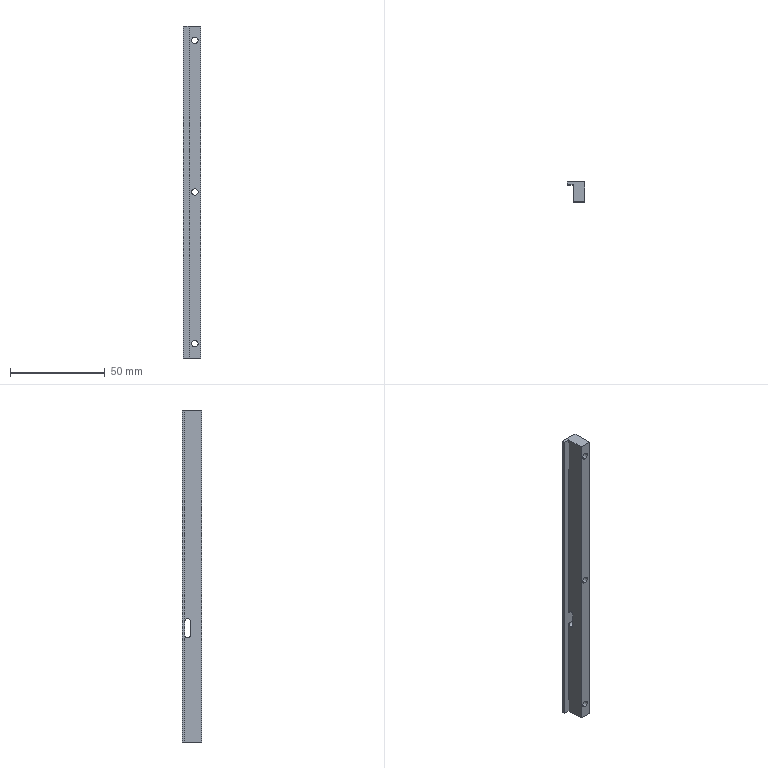Part | STEP file | PN_0021 | 1 solid | 19 faces | box 9 x 10.5 x 175 mm | volume 11358 mm3 | cylinder 10 | plane 9 | commonest cylinder face diameters 3.4 x6 3 x4
STEP:
#1=CARTESIAN_POINT('',(0.,0.,0.));
#2=DIRECTION('',(0.,0.,1.));
#3=DIRECTION('',(1.,0.,0.));
#4=AXIS2_PLACEMENT_3D('',#1,#2,#3);
#5=CARTESIAN_POINT('',(1.5,0.,-78.3));
#6=VERTEX_POINT('',#5);
#7=CARTESIAN_POINT('',(1.5,10.5,-78.3));
#8=VERTEX_POINT('',#7);
#9=CARTESIAN_POINT('',(1.5,10.5,-78.3));
#10=DIRECTION('',(0.,1.,0.));
#11=VECTOR('',#10,1.);
#12=LINE('',#9,#11);
#13=CARTESIAN_POINT('',(1.5,10.5,-80.));
#14=DIRECTION('',(0.,1.,0.));
#15=DIRECTION('',(0.,0.,1.));
#16=AXIS2_PLACEMENT_3D('',#13,#14,#15);
#17=CYLINDRICAL_SURFACE('',#16,1.7);
#18=CARTESIAN_POINT('',(6.283,0.));
#19=DIRECTION('',(0.,1.));
#20=VECTOR('',#19,1.);
#21=LINE('',#18,#20);
#22=(GEOMETRIC_REPRESENTATION_CONTEXT(2)PARAMETRIC_REPRESENTATION_CONTEXT()REPRESENTATION_CONTEXT('',''));
#23=DEFINITIONAL_REPRESENTATION('',(#21),#22);
#24=PCURVE('',#17,#23);
#25=CARTESIAN_POINT('',(1.5,10.5,-80.));
#26=DIRECTION('',(0.,1.,0.));
#27=DIRECTION('',(0.,0.,1.));
#28=AXIS2_PLACEMENT_3D('',#25,#26,#27);
#29=CYLINDRICAL_SURFACE('',#28,1.7);
#30=CARTESIAN_POINT('',(0.,0.));
#31=DIRECTION('',(0.,1.));
#32=VECTOR('',#31,1.);
#33=LINE('',#30,#32);
#34=(GEOMETRIC_REPRESENTATION_CONTEXT(2)PARAMETRIC_REPRESENTATION_CONTEXT()REPRESENTATION_CONTEXT('',''));
#35=DEFINITIONAL_REPRESENTATION('',(#33),#34);
#36=PCURVE('',#29,#35);
#37=SURFACE_CURVE('',#12,(#24,#36),.PCURVE_S1.);
#38=EDGE_CURVE('',#6,#8,#37,.T.);
#39=ORIENTED_EDGE('',*,*,#38,.T.);
#40=CARTESIAN_POINT('',(1.5,10.5,-81.7));
#41=VERTEX_POINT('',#40);
#42=CARTESIAN_POINT('',(1.5,10.5,-80.));
#43=DIRECTION('',(0.,1.,0.));
#44=DIRECTION('',(0.,0.,1.));
#45=AXIS2_PLACEMENT_3D('',#42,#43,#44);
#46=CIRCLE('',#45,1.7);
#47=CARTESIAN_POINT('',(0.,0.));
#48=DIRECTION('',(1.,0.));
#49=VECTOR('',#48,1.);
#50=LINE('',#47,#49);
#51=(GEOMETRIC_REPRESENTATION_CONTEXT(2)PARAMETRIC_REPRESENTATION_CONTEXT()REPRESENTATION_CONTEXT('',''));
#52=DEFINITIONAL_REPRESENTATION('',(#50),#51);
#53=PCURVE('',#17,#52);
#54=CARTESIAN_POINT('',(0.,10.5,0.));
#55=DIRECTION('',(0.,1.,0.));
#56=DIRECTION('',(0.,0.,1.));
#57=AXIS2_PLACEMENT_3D('',#54,#55,#56);
#58=PLANE('',#57);
#59=CARTESIAN_POINT('',(-80.,1.5));
#60=DIRECTION('',(1.,0.));
#61=AXIS2_PLACEMENT_2D('',#59,#60);
#62=CIRCLE('',#61,1.7);
#63=(GEOMETRIC_REPRESENTATION_CONTEXT(2)PARAMETRIC_REPRESENTATION_CONTEXT()REPRESENTATION_CONTEXT('',''));
#64=DEFINITIONAL_REPRESENTATION('',(#62),#63);
#65=PCURVE('',#58,#64);
#66=SURFACE_CURVE('',#46,(#53,#65),.PCURVE_S1.);
#67=EDGE_CURVE('',#41,#8,#66,.T.);
#68=ORIENTED_EDGE('',*,*,#67,.F.);
#69=CARTESIAN_POINT('',(1.5,0.,-81.7));
#70=VERTEX_POINT('',#69);
#71=CARTESIAN_POINT('',(1.5,10.5,-81.7));
#72=DIRECTION('',(0.,1.,0.));
#73=VECTOR('',#72,1.);
#74=LINE('',#71,#73);
#75=CARTESIAN_POINT('',(3.142,0.));
#76=DIRECTION('',(0.,1.));
#77=VECTOR('',#76,1.);
#78=LINE('',#75,#77);
#79=(GEOMETRIC_REPRESENTATION_CONTEXT(2)PARAMETRIC_REPRESENTATION_CONTEXT()REPRESENTATION_CONTEXT('',''));
#80=DEFINITIONAL_REPRESENTATION('',(#78),#79);
#81=PCURVE('',#17,#80);
#82=CARTESIAN_POINT('',(3.142,0.));
#83=DIRECTION('',(0.,1.));
#84=VECTOR('',#83,1.);
#85=LINE('',#82,#84);
#86=(GEOMETRIC_REPRESENTATION_CONTEXT(2)PARAMETRIC_REPRESENTATION_CONTEXT()REPRESENTATION_CONTEXT('',''));
#87=DEFINITIONAL_REPRESENTATION('',(#85),#86);
#88=PCURVE('',#29,#87);
#89=SURFACE_CURVE('',#74,(#81,#88),.PCURVE_S1.);
#90=EDGE_CURVE('',#70,#41,#89,.T.);
#91=ORIENTED_EDGE('',*,*,#90,.F.);
#92=CARTESIAN_POINT('',(1.5,0.,-80.));
#93=DIRECTION('',(0.,1.,0.));
#94=DIRECTION('',(0.,0.,1.));
#95=AXIS2_PLACEMENT_3D('',#92,#93,#94);
#96=CIRCLE('',#95,1.7);
#97=CARTESIAN_POINT('',(0.,-10.5));
#98=DIRECTION('',(1.,0.));
#99=VECTOR('',#98,1.);
#100=LINE('',#97,#99);
#101=(GEOMETRIC_REPRESENTATION_CONTEXT(2)PARAMETRIC_REPRESENTATION_CONTEXT()REPRESENTATION_CONTEXT('',''));
#102=DEFINITIONAL_REPRESENTATION('',(#100),#101);
#103=PCURVE('',#17,#102);
#104=CARTESIAN_POINT('',(0.,0.,0.));
#105=DIRECTION('',(0.,1.,0.));
#106=DIRECTION('',(0.,0.,1.));
#107=AXIS2_PLACEMENT_3D('',#104,#105,#106);
#108=PLANE('',#107);
#109=CARTESIAN_POINT('',(-80.,1.5));
#110=DIRECTION('',(1.,0.));
#111=AXIS2_PLACEMENT_2D('',#109,#110);
#112=CIRCLE('',#111,1.7);
#113=(GEOMETRIC_REPRESENTATION_CONTEXT(2)PARAMETRIC_REPRESENTATION_CONTEXT()REPRESENTATION_CONTEXT('',''));
#114=DEFINITIONAL_REPRESENTATION('',(#112),#113);
#115=PCURVE('',#108,#114);
#116=SURFACE_CURVE('',#96,(#103,#115),.PCURVE_S1.);
#117=EDGE_CURVE('',#70,#6,#116,.T.);
#118=ORIENTED_EDGE('',*,*,#117,.T.);
#119=EDGE_LOOP('',(#39,#68,#91,#118));
#120=FACE_BOUND('',#119,.F.);
#121=ADVANCED_FACE('',(#120),#17,.F.);
#122=CARTESIAN_POINT('',(1.5,0.,1.7));
#123=VERTEX_POINT('',#122);
#124=CARTESIAN_POINT('',(1.5,10.5,1.7));
#125=VERTEX_POINT('',#124);
#126=CARTESIAN_POINT('',(1.5,10.5,1.7));
#127=DIRECTION('',(0.,1.,0.));
#128=VECTOR('',#127,1.);
#129=LINE('',#126,#128);
#130=CARTESIAN_POINT('',(1.5,10.5,0.));
#131=DIRECTION('',(0.,1.,0.));
#132=DIRECTION('',(0.,0.,1.));
#133=AXIS2_PLACEMENT_3D('',#130,#131,#132);
#134=CYLINDRICAL_SURFACE('',#133,1.7);
#135=CARTESIAN_POINT('',(6.283,0.));
#136=DIRECTION('',(0.,1.));
#137=VECTOR('',#136,1.);
#138=LINE('',#135,#137);
#139=(GEOMETRIC_REPRESENTATION_CONTEXT(2)PARAMETRIC_REPRESENTATION_CONTEXT()REPRESENTATION_CONTEXT('',''));
#140=DEFINITIONAL_REPRESENTATION('',(#138),#139);
#141=PCURVE('',#134,#140);
#142=CARTESIAN_POINT('',(1.5,10.5,0.));
#143=DIRECTION('',(0.,1.,0.));
#144=DIRECTION('',(0.,0.,1.));
#145=AXIS2_PLACEMENT_3D('',#142,#143,#144);
#146=CYLINDRICAL_SURFACE('',#145,1.7);
#147=CARTESIAN_POINT('',(0.,0.));
#148=DIRECTION('',(0.,1.));
#149=VECTOR('',#148,1.);
#150=LINE('',#147,#149);
#151=(GEOMETRIC_REPRESENTATION_CONTEXT(2)PARAMETRIC_REPRESENTATION_CONTEXT()REPRESENTATION_CONTEXT('',''));
#152=DEFINITIONAL_REPRESENTATION('',(#150),#151);
#153=PCURVE('',#146,#152);
#154=SURFACE_CURVE('',#129,(#141,#153),.PCURVE_S1.);
#155=EDGE_CURVE('',#123,#125,#154,.T.);
#156=ORIENTED_EDGE('',*,*,#155,.T.);
#157=CARTESIAN_POINT('',(1.5,10.5,-1.7));
#158=VERTEX_POINT('',#157);
#159=CARTESIAN_POINT('',(1.5,10.5,0.));
#160=DIRECTION('',(0.,1.,0.));
#161=DIRECTION('',(0.,0.,1.));
#162=AXIS2_PLACEMENT_3D('',#159,#160,#161);
#163=CIRCLE('',#162,1.7);
#164=CARTESIAN_POINT('',(0.,0.));
#165=DIRECTION('',(1.,0.));
#166=VECTOR('',#165,1.);
#167=LINE('',#164,#166);
#168=(GEOMETRIC_REPRESENTATION_CONTEXT(2)PARAMETRIC_REPRESENTATION_CONTEXT()REPRESENTATION_CONTEXT('',''));
#169=DEFINITIONAL_REPRESENTATION('',(#167),#168);
#170=PCURVE('',#134,#169);
#171=CARTESIAN_POINT('',(0.,1.5));
#172=DIRECTION('',(1.,0.));
#173=AXIS2_PLACEMENT_2D('',#171,#172);
#174=CIRCLE('',#173,1.7);
#175=(GEOMETRIC_REPRESENTATION_CONTEXT(2)PARAMETRIC_REPRESENTATION_CONTEXT()REPRESENTATION_CONTEXT('',''));
#176=DEFINITIONAL_REPRESENTATION('',(#174),#175);
#177=PCURVE('',#58,#176);
#178=SURFACE_CURVE('',#163,(#170,#177),.PCURVE_S1.);
#179=EDGE_CURVE('',#158,#125,#178,.T.);
#180=ORIENTED_EDGE('',*,*,#179,.F.);
#181=CARTESIAN_POINT('',(1.5,0.,-1.7));
#182=VERTEX_POINT('',#181);
#183=CARTESIAN_POINT('',(1.5,10.5,-1.7));
#184=DIRECTION('',(0.,1.,0.));
#185=VECTOR('',#184,1.);
#186=LINE('',#183,#185);
#187=CARTESIAN_POINT('',(3.142,0.));
#188=DIRECTION('',(0.,1.));
#189=VECTOR('',#188,1.);
#190=LINE('',#187,#189);
#191=(GEOMETRIC_REPRESENTATION_CONTEXT(2)PARAMETRIC_REPRESENTATION_CONTEXT()REPRESENTATION_CONTEXT('',''));
#192=DEFINITIONAL_REPRESENTATION('',(#190),#191);
#193=PCURVE('',#134,#192);
#194=CARTESIAN_POINT('',(3.142,0.));
#195=DIRECTION('',(0.,1.));
#196=VECTOR('',#195,1.);
#197=LINE('',#194,#196);
#198=(GEOMETRIC_REPRESENTATION_CONTEXT(2)PARAMETRIC_REPRESENTATION_CONTEXT()REPRESENTATION_CONTEXT('',''));
#199=DEFINITIONAL_REPRESENTATION('',(#197),#198);
#200=PCURVE('',#146,#199);
#201=SURFACE_CURVE('',#186,(#193,#200),.PCURVE_S1.);
#202=EDGE_CURVE('',#182,#158,#201,.T.);
#203=ORIENTED_EDGE('',*,*,#202,.F.);
#204=CARTESIAN_POINT('',(1.5,0.,0.));
#205=DIRECTION('',(0.,1.,0.));
#206=DIRECTION('',(0.,0.,1.));
#207=AXIS2_PLACEMENT_3D('',#204,#205,#206);
#208=CIRCLE('',#207,1.7);
#209=CARTESIAN_POINT('',(0.,-10.5));
#210=DIRECTION('',(1.,0.));
#211=VECTOR('',#210,1.);
#212=LINE('',#209,#211);
#213=(GEOMETRIC_REPRESENTATION_CONTEXT(2)PARAMETRIC_REPRESENTATION_CONTEXT()REPRESENTATION_CONTEXT('',''));
#214=DEFINITIONAL_REPRESENTATION('',(#212),#213);
#215=PCURVE('',#134,#214);
#216=CARTESIAN_POINT('',(0.,1.5));
#217=DIRECTION('',(1.,0.));
#218=AXIS2_PLACEMENT_2D('',#216,#217);
#219=CIRCLE('',#218,1.7);
#220=(GEOMETRIC_REPRESENTATION_CONTEXT(2)PARAMETRIC_REPRESENTATION_CONTEXT()REPRESENTATION_CONTEXT('',''));
#221=DEFINITIONAL_REPRESENTATION('',(#219),#220);
#222=PCURVE('',#108,#221);
#223=SURFACE_CURVE('',#208,(#215,#222),.PCURVE_S1.);
#224=EDGE_CURVE('',#182,#123,#223,.T.);
#225=ORIENTED_EDGE('',*,*,#224,.T.);
#226=EDGE_LOOP('',(#156,#180,#203,#225));
#227=FACE_BOUND('',#226,.F.);
#228=ADVANCED_FACE('',(#227),#134,.F.);
#229=CARTESIAN_POINT('',(1.5,0.,81.7));
#230=VERTEX_POINT('',#229);
#231=CARTESIAN_POINT('',(1.5,10.5,81.7));
#232=VERTEX_POINT('',#231);
#233=CARTESIAN_POINT('',(1.5,10.5,81.7));
#234=DIRECTION('',(0.,1.,0.));
#235=VECTOR('',#234,1.);
#236=LINE('',#233,#235);
#237=CARTESIAN_POINT('',(1.5,10.5,80.));
#238=DIRECTION('',(0.,1.,0.));
#239=DIRECTION('',(0.,0.,1.));
#240=AXIS2_PLACEMENT_3D('',#237,#238,#239);
#241=CYLINDRICAL_SURFACE('',#240,1.7);
#242=CARTESIAN_POINT('',(6.283,0.));
#243=DIRECTION('',(0.,1.));
#244=VECTOR('',#243,1.);
#245=LINE('',#242,#244);
#246=(GEOMETRIC_REPRESENTATION_CONTEXT(2)PARAMETRIC_REPRESENTATION_CONTEXT()REPRESENTATION_CONTEXT('',''));
#247=DEFINITIONAL_REPRESENTATION('',(#245),#246);
#248=PCURVE('',#241,#247);
#249=CARTESIAN_POINT('',(1.5,10.5,80.));
#250=DIRECTION('',(0.,1.,0.));
#251=DIRECTION('',(0.,0.,1.));
#252=AXIS2_PLACEMENT_3D('',#249,#250,#251);
#253=CYLINDRICAL_SURFACE('',#252,1.7);
#254=CARTESIAN_POINT('',(0.,0.));
#255=DIRECTION('',(0.,1.));
#256=VECTOR('',#255,1.);
#257=LINE('',#254,#256);
#258=(GEOMETRIC_REPRESENTATION_CONTEXT(2)PARAMETRIC_REPRESENTATION_CONTEXT()REPRESENTATION_CONTEXT('',''));
#259=DEFINITIONAL_REPRESENTATION('',(#257),#258);
#260=PCURVE('',#253,#259);
#261=SURFACE_CURVE('',#236,(#248,#260),.PCURVE_S1.);
#262=EDGE_CURVE('',#230,#232,#261,.T.);
#263=ORIENTED_EDGE('',*,*,#262,.T.);
#264=CARTESIAN_POINT('',(1.5,10.5,78.3));
#265=VERTEX_POINT('',#264);
#266=CARTESIAN_POINT('',(1.5,10.5,80.));
#267=DIRECTION('',(0.,1.,0.));
#268=DIRECTION('',(0.,0.,1.));
#269=AXIS2_PLACEMENT_3D('',#266,#267,#268);
#270=CIRCLE('',#269,1.7);
#271=CARTESIAN_POINT('',(0.,0.));
#272=DIRECTION('',(1.,0.));
#273=VECTOR('',#272,1.);
#274=LINE('',#271,#273);
#275=(GEOMETRIC_REPRESENTATION_CONTEXT(2)PARAMETRIC_REPRESENTATION_CONTEXT()REPRESENTATION_CONTEXT('',''));
#276=DEFINITIONAL_REPRESENTATION('',(#274),#275);
#277=PCURVE('',#241,#276);
#278=CARTESIAN_POINT('',(80.,1.5));
#279=DIRECTION('',(1.,0.));
#280=AXIS2_PLACEMENT_2D('',#278,#279);
#281=CIRCLE('',#280,1.7);
#282=(GEOMETRIC_REPRESENTATION_CONTEXT(2)PARAMETRIC_REPRESENTATION_CONTEXT()REPRESENTATION_CONTEXT('',''));
#283=DEFINITIONAL_REPRESENTATION('',(#281),#282);
#284=PCURVE('',#58,#283);
#285=SURFACE_CURVE('',#270,(#277,#284),.PCURVE_S1.);
#286=EDGE_CURVE('',#265,#232,#285,.T.);
#287=ORIENTED_EDGE('',*,*,#286,.F.);
#288=CARTESIAN_POINT('',(1.5,0.,78.3));
#289=VERTEX_POINT('',#288);
#290=CARTESIAN_POINT('',(1.5,10.5,78.3));
#291=DIRECTION('',(0.,1.,0.));
#292=VECTOR('',#291,1.);
#293=LINE('',#290,#292);
#294=CARTESIAN_POINT('',(3.142,0.));
#295=DIRECTION('',(0.,1.));
#296=VECTOR('',#295,1.);
#297=LINE('',#294,#296);
#298=(GEOMETRIC_REPRESENTATION_CONTEXT(2)PARAMETRIC_REPRESENTATION_CONTEXT()REPRESENTATION_CONTEXT('',''));
#299=DEFINITIONAL_REPRESENTATION('',(#297),#298);
#300=PCURVE('',#241,#299);
#301=CARTESIAN_POINT('',(3.142,0.));
#302=DIRECTION('',(0.,1.));
#303=VECTOR('',#302,1.);
#304=LINE('',#301,#303);
#305=(GEOMETRIC_REPRESENTATION_CONTEXT(2)PARAMETRIC_REPRESENTATION_CONTEXT()REPRESENTATION_CONTEXT('',''));
#306=DEFINITIONAL_REPRESENTATION('',(#304),#305);
#307=PCURVE('',#253,#306);
#308=SURFACE_CURVE('',#293,(#300,#307),.PCURVE_S1.);
#309=EDGE_CURVE('',#289,#265,#308,.T.);
#310=ORIENTED_EDGE('',*,*,#309,.F.);
#311=CARTESIAN_POINT('',(1.5,0.,80.));
#312=DIRECTION('',(0.,1.,0.));
#313=DIRECTION('',(0.,0.,1.));
#314=AXIS2_PLACEMENT_3D('',#311,#312,#313);
#315=CIRCLE('',#314,1.7);
#316=CARTESIAN_POINT('',(0.,-10.5));
#317=DIRECTION('',(1.,0.));
#318=VECTOR('',#317,1.);
#319=LINE('',#316,#318);
#320=(GEOMETRIC_REPRESENTATION_CONTEXT(2)PARAMETRIC_REPRESENTATION_CONTEXT()REPRESENTATION_CONTEXT('',''));
#321=DEFINITIONAL_REPRESENTATION('',(#319),#320);
#322=PCURVE('',#241,#321);
#323=CARTESIAN_POINT('',(80.,1.5));
#324=DIRECTION('',(1.,0.));
#325=AXIS2_PLACEMENT_2D('',#323,#324);
#326=CIRCLE('',#325,1.7);
#327=(GEOMETRIC_REPRESENTATION_CONTEXT(2)PARAMETRIC_REPRESENTATION_CONTEXT()REPRESENTATION_CONTEXT('',''));
#328=DEFINITIONAL_REPRESENTATION('',(#326),#327);
#329=PCURVE('',#108,#328);
#330=SURFACE_CURVE('',#315,(#322,#329),.PCURVE_S1.);
#331=EDGE_CURVE('',#289,#230,#330,.T.);
#332=ORIENTED_EDGE('',*,*,#331,.T.);
#333=EDGE_LOOP('',(#263,#287,#310,#332));
#334=FACE_BOUND('',#333,.F.);
#335=ADVANCED_FACE('',(#334),#241,.F.);
#336=CARTESIAN_POINT('',(4.5,6.,-24.));
#337=VERTEX_POINT('',#336);
#338=CARTESIAN_POINT('',(4.5,7.5,-22.5));
#339=VERTEX_POINT('',#338);
#340=CARTESIAN_POINT('',(4.5,7.5,-24.));
#341=DIRECTION('',(-1.,0.,0.));
#342=DIRECTION('',(0.,0.,1.));
#343=AXIS2_PLACEMENT_3D('',#340,#341,#342);
#344=CIRCLE('',#343,1.5);
#345=CARTESIAN_POINT('',(4.5,10.5,-87.5));
#346=DIRECTION('',(-1.,0.,0.));
#347=DIRECTION('',(0.,0.,1.));
#348=AXIS2_PLACEMENT_3D('',#345,#346,#347);
#349=PLANE('',#348);
#350=CARTESIAN_POINT('',(63.5,-3.));
#351=DIRECTION('',(1.,0.));
#352=AXIS2_PLACEMENT_2D('',#350,#351);
#353=CIRCLE('',#352,1.5);
#354=(GEOMETRIC_REPRESENTATION_CONTEXT(2)PARAMETRIC_REPRESENTATION_CONTEXT()REPRESENTATION_CONTEXT('',''));
#355=DEFINITIONAL_REPRESENTATION('',(#353),#354);
#356=PCURVE('',#349,#355);
#357=CARTESIAN_POINT('',(4.5,7.5,-24.));
#358=DIRECTION('',(1.,0.,0.));
#359=DIRECTION('',(0.,0.,-1.));
#360=AXIS2_PLACEMENT_3D('',#357,#358,#359);
#361=CYLINDRICAL_SURFACE('',#360,1.5);
#362=CARTESIAN_POINT('',(9.425,0.));
#363=DIRECTION('',(-1.,0.));
#364=VECTOR('',#363,1.);
#365=LINE('',#362,#364);
#366=(GEOMETRIC_REPRESENTATION_CONTEXT(2)PARAMETRIC_REPRESENTATION_CONTEXT()REPRESENTATION_CONTEXT('',''));
#367=DEFINITIONAL_REPRESENTATION('',(#365),#366);
#368=PCURVE('',#361,#367);
#369=SURFACE_CURVE('',#344,(#356,#368),.PCURVE_S1.);
#370=EDGE_CURVE('',#337,#339,#369,.T.);
#371=ORIENTED_EDGE('',*,*,#370,.T.);
#372=CARTESIAN_POINT('',(4.5,9.,-24.));
#373=VERTEX_POINT('',#372);
#374=CARTESIAN_POINT('',(4.5,7.5,-24.));
#375=DIRECTION('',(-1.,0.,0.));
#376=DIRECTION('',(0.,0.,1.));
#377=AXIS2_PLACEMENT_3D('',#374,#375,#376);
#378=CIRCLE('',#377,1.5);
#379=CARTESIAN_POINT('',(63.5,-3.));
#380=DIRECTION('',(1.,0.));
#381=AXIS2_PLACEMENT_2D('',#379,#380);
#382=CIRCLE('',#381,1.5);
#383=(GEOMETRIC_REPRESENTATION_CONTEXT(2)PARAMETRIC_REPRESENTATION_CONTEXT()REPRESENTATION_CONTEXT('',''));
#384=DEFINITIONAL_REPRESENTATION('',(#382),#383);
#385=PCURVE('',#349,#384);
#386=CARTESIAN_POINT('',(-4.5,7.5,-24.));
#387=DIRECTION('',(1.,0.,0.));
#388=DIRECTION('',(0.,0.,-1.));
#389=AXIS2_PLACEMENT_3D('',#386,#387,#388);
#390=CYLINDRICAL_SURFACE('',#389,1.5);
#391=CARTESIAN_POINT('',(3.142,9.));
#392=DIRECTION('',(-1.,0.));
#393=VECTOR('',#392,1.);
#394=LINE('',#391,#393);
#395=(GEOMETRIC_REPRESENTATION_CONTEXT(2)PARAMETRIC_REPRESENTATION_CONTEXT()REPRESENTATION_CONTEXT('',''));
#396=DEFINITIONAL_REPRESENTATION('',(#394),#395);
#397=PCURVE('',#390,#396);
#398=SURFACE_CURVE('',#378,(#385,#397),.PCURVE_S1.);
#399=EDGE_CURVE('',#339,#373,#398,.T.);
#400=ORIENTED_EDGE('',*,*,#399,.T.);
#401=CARTESIAN_POINT('',(4.5,9.,-31.));
#402=VERTEX_POINT('',#401);
#403=CARTESIAN_POINT('',(4.5,9.,-32.5));
#404=DIRECTION('',(0.,0.,-1.));
#405=VECTOR('',#404,1.);
#406=LINE('',#403,#405);
#407=CARTESIAN_POINT('',(55.,-1.5));
#408=DIRECTION('',(-1.,0.));
#409=VECTOR('',#408,1.);
#410=LINE('',#407,#409);
#411=(GEOMETRIC_REPRESENTATION_CONTEXT(2)PARAMETRIC_REPRESENTATION_CONTEXT()REPRESENTATION_CONTEXT('',''));
#412=DEFINITIONAL_REPRESENTATION('',(#410),#411);
#413=PCURVE('',#349,#412);
#414=CARTESIAN_POINT('',(-4.5,9.,-87.5));
#415=DIRECTION('',(0.,1.,0.));
#416=DIRECTION('',(0.,0.,1.));
#417=AXIS2_PLACEMENT_3D('',#414,#415,#416);
#418=PLANE('',#417);
#419=CARTESIAN_POINT('',(55.,9.));
#420=DIRECTION('',(-1.,0.));
#421=VECTOR('',#420,1.);
#422=LINE('',#419,#421);
#423=(GEOMETRIC_REPRESENTATION_CONTEXT(2)PARAMETRIC_REPRESENTATION_CONTEXT()REPRESENTATION_CONTEXT('',''));
#424=DEFINITIONAL_REPRESENTATION('',(#422),#423);
#425=PCURVE('',#418,#424);
#426=SURFACE_CURVE('',#406,(#413,#425),.PCURVE_S1.);
#427=EDGE_CURVE('',#373,#402,#426,.T.);
#428=ORIENTED_EDGE('',*,*,#427,.T.);
#429=CARTESIAN_POINT('',(4.5,7.5,-32.5));
#430=VERTEX_POINT('',#429);
#431=CARTESIAN_POINT('',(4.5,7.5,-31.));
#432=DIRECTION('',(-1.,0.,0.));
#433=DIRECTION('',(0.,0.,1.));
#434=AXIS2_PLACEMENT_3D('',#431,#432,#433);
#435=CIRCLE('',#434,1.5);
#436=CARTESIAN_POINT('',(56.5,-3.));
#437=DIRECTION('',(1.,0.));
#438=AXIS2_PLACEMENT_2D('',#436,#437);
#439=CIRCLE('',#438,1.5);
#440=(GEOMETRIC_REPRESENTATION_CONTEXT(2)PARAMETRIC_REPRESENTATION_CONTEXT()REPRESENTATION_CONTEXT('',''));
#441=DEFINITIONAL_REPRESENTATION('',(#439),#440);
#442=PCURVE('',#349,#441);
#443=CARTESIAN_POINT('',(4.5,7.5,-31.));
#444=DIRECTION('',(1.,0.,0.));
#445=DIRECTION('',(0.,0.,-1.));
#446=AXIS2_PLACEMENT_3D('',#443,#444,#445);
#447=CYLINDRICAL_SURFACE('',#446,1.5);
#448=CARTESIAN_POINT('',(3.142,0.));
#449=DIRECTION('',(-1.,0.));
#450=VECTOR('',#449,1.);
#451=LINE('',#448,#450);
#452=(GEOMETRIC_REPRESENTATION_CONTEXT(2)PARAMETRIC_REPRESENTATION_CONTEXT()REPRESENTATION_CONTEXT('',''));
#453=DEFINITIONAL_REPRESENTATION('',(#451),#452);
#454=PCURVE('',#447,#453);
#455=SURFACE_CURVE('',#435,(#442,#454),.PCURVE_S1.);
#456=EDGE_CURVE('',#402,#430,#455,.T.);
#457=ORIENTED_EDGE('',*,*,#456,.T.);
#458=CARTESIAN_POINT('',(4.5,6.,-31.));
#459=VERTEX_POINT('',#458);
#460=CARTESIAN_POINT('',(4.5,7.5,-31.));
#461=DIRECTION('',(-1.,0.,0.));
#462=DIRECTION('',(0.,0.,1.));
#463=AXIS2_PLACEMENT_3D('',#460,#461,#462);
#464=CIRCLE('',#463,1.5);
#465=CARTESIAN_POINT('',(56.5,-3.));
#466=DIRECTION('',(1.,0.));
#467=AXIS2_PLACEMENT_2D('',#465,#466);
#468=CIRCLE('',#467,1.5);
#469=(GEOMETRIC_REPRESENTATION_CONTEXT(2)PARAMETRIC_REPRESENTATION_CONTEXT()REPRESENTATION_CONTEXT('',''));
#470=DEFINITIONAL_REPRESENTATION('',(#468),#469);
#471=PCURVE('',#349,#470);
#472=CARTESIAN_POINT('',(4.5,7.5,-31.));
#473=DIRECTION('',(1.,0.,0.));
#474=DIRECTION('',(0.,0.,-1.));
#475=AXIS2_PLACEMENT_3D('',#472,#473,#474);
#476=CYLINDRICAL_SURFACE('',#475,1.5);
#477=CARTESIAN_POINT('',(9.425,0.));
#478=DIRECTION('',(-1.,0.));
#479=VECTOR('',#478,1.);
#480=LINE('',#477,#479);
#481=(GEOMETRIC_REPRESENTATION_CONTEXT(2)PARAMETRIC_REPRESENTATION_CONTEXT()REPRESENTATION_CONTEXT('',''));
#482=DEFINITIONAL_REPRESENTATION('',(#480),#481);
#483=PCURVE('',#476,#482);
#484=SURFACE_CURVE('',#464,(#471,#483),.PCURVE_S1.);
#485=EDGE_CURVE('',#430,#459,#484,.T.);
#486=ORIENTED_EDGE('',*,*,#485,.T.);
#487=CARTESIAN_POINT('',(4.5,6.,-32.5));
#488=DIRECTION('',(0.,0.,1.));
#489=VECTOR('',#488,1.);
#490=LINE('',#487,#489);
#491=CARTESIAN_POINT('',(55.,-4.5));
#492=DIRECTION('',(1.,0.));
#493=VECTOR('',#492,1.);
#494=LINE('',#491,#493);
#495=(GEOMETRIC_REPRESENTATION_CONTEXT(2)PARAMETRIC_REPRESENTATION_CONTEXT()REPRESENTATION_CONTEXT('',''));
#496=DEFINITIONAL_REPRESENTATION('',(#494),#495);
#497=PCURVE('',#349,#496);
#498=CARTESIAN_POINT('',(4.5,6.,-32.5));
#499=DIRECTION('',(0.,-1.,0.));
#500=DIRECTION('',(0.,0.,-1.));
#501=AXIS2_PLACEMENT_3D('',#498,#499,#500);
#502=PLANE('',#501);
#503=CARTESIAN_POINT('',(0.,0.));
#504=DIRECTION('',(-1.,0.));
#505=VECTOR('',#504,1.);
#506=LINE('',#503,#505);
#507=(GEOMETRIC_REPRESENTATION_CONTEXT(2)PARAMETRIC_REPRESENTATION_CONTEXT()REPRESENTATION_CONTEXT('',''));
#508=DEFINITIONAL_REPRESENTATION('',(#506),#507);
#509=PCURVE('',#502,#508);
#510=SURFACE_CURVE('',#490,(#497,#509),.PCURVE_S1.);
#511=EDGE_CURVE('',#459,#337,#510,.T.);
#512=ORIENTED_EDGE('',*,*,#511,.T.);
#513=EDGE_LOOP('',(#371,#400,#428,#457,#486,#512));
#514=FACE_BOUND('',#513,.T.);
#515=CARTESIAN_POINT('',(4.5,0.,87.5));
#516=VERTEX_POINT('',#515);
#517=CARTESIAN_POINT('',(4.5,0.,-87.5));
#518=VERTEX_POINT('',#517);
#519=CARTESIAN_POINT('',(4.5,0.,-87.5));
#520=DIRECTION('',(0.,0.,-1.));
#521=VECTOR('',#520,1.);
#522=LINE('',#519,#521);
#523=CARTESIAN_POINT('',(0.,-10.5));
#524=DIRECTION('',(-1.,0.));
#525=VECTOR('',#524,1.);
#526=LINE('',#523,#525);
#527=(GEOMETRIC_REPRESENTATION_CONTEXT(2)PARAMETRIC_REPRESENTATION_CONTEXT()REPRESENTATION_CONTEXT('',''));
#528=DEFINITIONAL_REPRESENTATION('',(#526),#527);
#529=PCURVE('',#349,#528);
#530=CARTESIAN_POINT('',(-87.5,4.5));
#531=DIRECTION('',(-1.,0.));
#532=VECTOR('',#531,1.);
#533=LINE('',#530,#532);
#534=(GEOMETRIC_REPRESENTATION_CONTEXT(2)PARAMETRIC_REPRESENTATION_CONTEXT()REPRESENTATION_CONTEXT('',''));
#535=DEFINITIONAL_REPRESENTATION('',(#533),#534);
#536=PCURVE('',#108,#535);
#537=SURFACE_CURVE('',#522,(#529,#536),.PCURVE_S1.);
#538=EDGE_CURVE('',#516,#518,#537,.T.);
#539=ORIENTED_EDGE('',*,*,#538,.T.);
#540=CARTESIAN_POINT('',(4.5,10.5,-87.5));
#541=VERTEX_POINT('',#540);
#542=CARTESIAN_POINT('',(4.5,10.5,-87.5));
#543=DIRECTION('',(0.,-1.,0.));
#544=VECTOR('',#543,1.);
#545=LINE('',#542,#544);
#546=CARTESIAN_POINT('',(0.,0.));
#547=DIRECTION('',(0.,-1.));
#548=VECTOR('',#547,1.);
#549=LINE('',#546,#548);
#550=(GEOMETRIC_REPRESENTATION_CONTEXT(2)PARAMETRIC_REPRESENTATION_CONTEXT()REPRESENTATION_CONTEXT('',''));
#551=DEFINITIONAL_REPRESENTATION('',(#549),#550);
#552=PCURVE('',#349,#551);
#553=CARTESIAN_POINT('',(-4.5,10.5,-87.5));
#554=DIRECTION('',(0.,0.,1.));
#555=DIRECTION('',(1.,0.,0.));
#556=AXIS2_PLACEMENT_3D('',#553,#554,#555);
#557=PLANE('',#556);
#558=CARTESIAN_POINT('',(9.,0.));
#559=DIRECTION('',(0.,-1.));
#560=VECTOR('',#559,1.);
#561=LINE('',#558,#560);
#562=(GEOMETRIC_REPRESENTATION_CONTEXT(2)PARAMETRIC_REPRESENTATION_CONTEXT()REPRESENTATION_CONTEXT('',''));
#563=DEFINITIONAL_REPRESENTATION('',(#561),#562);
#564=PCURVE('',#557,#563);
#565=SURFACE_CURVE('',#545,(#552,#564),.PCURVE_S1.);
#566=EDGE_CURVE('',#541,#518,#565,.T.);
#567=ORIENTED_EDGE('',*,*,#566,.F.);
#568=CARTESIAN_POINT('',(4.5,10.5,87.5));
#569=VERTEX_POINT('',#568);
#570=CARTESIAN_POINT('',(4.5,10.5,-87.5));
#571=DIRECTION('',(0.,0.,-1.));
#572=VECTOR('',#571,1.);
#573=LINE('',#570,#572);
#574=CARTESIAN_POINT('',(0.,0.));
#575=DIRECTION('',(-1.,0.));
#576=VECTOR('',#575,1.);
#577=LINE('',#574,#576);
#578=(GEOMETRIC_REPRESENTATION_CONTEXT(2)PARAMETRIC_REPRESENTATION_CONTEXT()REPRESENTATION_CONTEXT('',''));
#579=DEFINITIONAL_REPRESENTATION('',(#577),#578);
#580=PCURVE('',#349,#579);
#581=CARTESIAN_POINT('',(-87.5,4.5));
#582=DIRECTION('',(-1.,0.));
#583=VECTOR('',#582,1.);
#584=LINE('',#581,#583);
#585=(GEOMETRIC_REPRESENTATION_CONTEXT(2)PARAMETRIC_REPRESENTATION_CONTEXT()REPRESENTATION_CONTEXT('',''));
#586=DEFINITIONAL_REPRESENTATION('',(#584),#585);
#587=PCURVE('',#58,#586);
#588=SURFACE_CURVE('',#573,(#580,#587),.PCURVE_S1.);
#589=EDGE_CURVE('',#569,#541,#588,.T.);
#590=ORIENTED_EDGE('',*,*,#589,.F.);
#591=CARTESIAN_POINT('',(4.5,10.5,87.5));
#592=DIRECTION('',(0.,-1.,0.));
#593=VECTOR('',#592,1.);
#594=LINE('',#591,#593);
#595=CARTESIAN_POINT('',(175.,0.));
#596=DIRECTION('',(0.,-1.));
#597=VECTOR('',#596,1.);
#598=LINE('',#595,#597);
#599=(GEOMETRIC_REPRESENTATION_CONTEXT(2)PARAMETRIC_REPRESENTATION_CONTEXT()REPRESENTATION_CONTEXT('',''));
#600=DEFINITIONAL_REPRESENTATION('',(#598),#599);
#601=PCURVE('',#349,#600);
#602=CARTESIAN_POINT('',(-4.5,10.5,87.5));
#603=DIRECTION('',(0.,0.,-1.));
#604=DIRECTION('',(-1.,0.,0.));
#605=AXIS2_PLACEMENT_3D('',#602,#603,#604);
#606=PLANE('',#605);
#607=CARTESIAN_POINT('',(-9.,0.));
#608=DIRECTION('',(0.,-1.));
#609=VECTOR('',#608,1.);
#610=LINE('',#607,#609);
#611=(GEOMETRIC_REPRESENTATION_CONTEXT(2)PARAMETRIC_REPRESENTATION_CONTEXT()REPRESENTATION_CONTEXT('',''));
#612=DEFINITIONAL_REPRESENTATION('',(#610),#611);
#613=PCURVE('',#606,#612);
#614=SURFACE_CURVE('',#594,(#601,#613),.PCURVE_S1.);
#615=EDGE_CURVE('',#569,#516,#614,.T.);
#616=ORIENTED_EDGE('',*,*,#615,.T.);
#617=EDGE_LOOP('',(#539,#567,#590,#616));
#618=FACE_BOUND('',#617,.T.);
#619=ADVANCED_FACE('',(#514,#618),#349,.F.);
#620=CARTESIAN_POINT('',(-1.5,0.,-87.5));
#621=VERTEX_POINT('',#620);
#622=CARTESIAN_POINT('',(-1.5,9.,-87.5));
#623=VERTEX_POINT('',#622);
#624=CARTESIAN_POINT('',(-1.5,0.,-87.5));
#625=DIRECTION('',(0.,1.,0.));
#626=VECTOR('',#625,1.);
#627=LINE('',#624,#626);
#628=CARTESIAN_POINT('',(3.,-10.5));
#629=DIRECTION('',(0.,1.));
#630=VECTOR('',#629,1.);
#631=LINE('',#628,#630);
#632=(GEOMETRIC_REPRESENTATION_CONTEXT(2)PARAMETRIC_REPRESENTATION_CONTEXT()REPRESENTATION_CONTEXT('',''));
#633=DEFINITIONAL_REPRESENTATION('',(#631),#632);
#634=PCURVE('',#557,#633);
#635=CARTESIAN_POINT('',(-1.5,0.,-87.5));
#636=DIRECTION('',(1.,0.,0.));
#637=DIRECTION('',(0.,0.,-1.));
#638=AXIS2_PLACEMENT_3D('',#635,#636,#637);
#639=PLANE('',#638);
#640=CARTESIAN_POINT('',(0.,0.));
#641=DIRECTION('',(0.,1.));
#642=VECTOR('',#641,1.);
#643=LINE('',#640,#642);
#644=(GEOMETRIC_REPRESENTATION_CONTEXT(2)PARAMETRIC_REPRESENTATION_CONTEXT()REPRESENTATION_CONTEXT('',''));
#645=DEFINITIONAL_REPRESENTATION('',(#643),#644);
#646=PCURVE('',#639,#645);
#647=SURFACE_CURVE('',#627,(#634,#646),.PCURVE_S1.);
#648=EDGE_CURVE('',#621,#623,#647,.T.);
#649=ORIENTED_EDGE('',*,*,#648,.T.);
#650=CARTESIAN_POINT('',(-4.5,9.,-87.5));
#651=VERTEX_POINT('',#650);
#652=CARTESIAN_POINT('',(-4.5,9.,-87.5));
#653=DIRECTION('',(-1.,0.,0.));
#654=VECTOR('',#653,1.);
#655=LINE('',#652,#654);
#656=CARTESIAN_POINT('',(0.,-1.5));
#657=DIRECTION('',(-1.,0.));
#658=VECTOR('',#657,1.);
#659=LINE('',#656,#658);
#660=(GEOMETRIC_REPRESENTATION_CONTEXT(2)PARAMETRIC_REPRESENTATION_CONTEXT()REPRESENTATION_CONTEXT('',''));
#661=DEFINITIONAL_REPRESENTATION('',(#659),#660);
#662=PCURVE('',#557,#661);
#663=CARTESIAN_POINT('',(0.,0.));
#664=DIRECTION('',(0.,-1.));
#665=VECTOR('',#664,1.);
#666=LINE('',#663,#665);
#667=(GEOMETRIC_REPRESENTATION_CONTEXT(2)PARAMETRIC_REPRESENTATION_CONTEXT()REPRESENTATION_CONTEXT('',''));
#668=DEFINITIONAL_REPRESENTATION('',(#666),#667);
#669=PCURVE('',#418,#668);
#670=SURFACE_CURVE('',#655,(#662,#669),.PCURVE_S1.);
#671=EDGE_CURVE('',#623,#651,#670,.T.);
#672=ORIENTED_EDGE('',*,*,#671,.T.);
#673=CARTESIAN_POINT('',(-4.5,10.5,-87.5));
#674=VERTEX_POINT('',#673);
#675=CARTESIAN_POINT('',(-4.5,10.5,-87.5));
#676=DIRECTION('',(0.,-1.,0.));
#677=VECTOR('',#676,1.);
#678=LINE('',#675,#677);
#679=CARTESIAN_POINT('',(0.,0.));
#680=DIRECTION('',(0.,-1.));
#681=VECTOR('',#680,1.);
#682=LINE('',#679,#681);
#683=(GEOMETRIC_REPRESENTATION_CONTEXT(2)PARAMETRIC_REPRESENTATION_CONTEXT()REPRESENTATION_CONTEXT('',''));
#684=DEFINITIONAL_REPRESENTATION('',(#682),#683);
#685=PCURVE('',#557,#684);
#686=CARTESIAN_POINT('',(-4.5,10.5,-87.5));
#687=DIRECTION('',(1.,0.,0.));
#688=DIRECTION('',(0.,0.,-1.));
#689=AXIS2_PLACEMENT_3D('',#686,#687,#688);
#690=PLANE('',#689);
#691=CARTESIAN_POINT('',(0.,0.));
#692=DIRECTION('',(0.,-1.));
#693=VECTOR('',#692,1.);
#694=LINE('',#691,#693);
#695=(GEOMETRIC_REPRESENTATION_CONTEXT(2)PARAMETRIC_REPRESENTATION_CONTEXT()REPRESENTATION_CONTEXT('',''));
#696=DEFINITIONAL_REPRESENTATION('',(#694),#695);
#697=PCURVE('',#690,#696);
#698=SURFACE_CURVE('',#678,(#685,#697),.PCURVE_S1.);
#699=EDGE_CURVE('',#674,#651,#698,.T.);
#700=ORIENTED_EDGE('',*,*,#699,.F.);
#701=CARTESIAN_POINT('',(-4.5,10.5,-87.5));
#702=DIRECTION('',(-1.,0.,0.));
#703=VECTOR('',#702,1.);
#704=LINE('',#701,#703);
#705=CARTESIAN_POINT('',(0.,0.));
#706=DIRECTION('',(-1.,0.));
#707=VECTOR('',#706,1.);
#708=LINE('',#705,#707);
#709=(GEOMETRIC_REPRESENTATION_CONTEXT(2)PARAMETRIC_REPRESENTATION_CONTEXT()REPRESENTATION_CONTEXT('',''));
#710=DEFINITIONAL_REPRESENTATION('',(#708),#709);
#711=PCURVE('',#557,#710);
#712=CARTESIAN_POINT('',(-87.5,-4.5));
#713=DIRECTION('',(0.,-1.));
#714=VECTOR('',#713,1.);
#715=LINE('',#712,#714);
#716=(GEOMETRIC_REPRESENTATION_CONTEXT(2)PARAMETRIC_REPRESENTATION_CONTEXT()REPRESENTATION_CONTEXT('',''));
#717=DEFINITIONAL_REPRESENTATION('',(#715),#716);
#718=PCURVE('',#58,#717);
#719=SURFACE_CURVE('',#704,(#711,#718),.PCURVE_S1.);
#720=EDGE_CURVE('',#541,#674,#719,.T.);
#721=ORIENTED_EDGE('',*,*,#720,.F.);
#722=ORIENTED_EDGE('',*,*,#566,.T.);
#723=CARTESIAN_POINT('',(-4.5,0.,-87.5));
#724=DIRECTION('',(-1.,0.,0.));
#725=VECTOR('',#724,1.);
#726=LINE('',#723,#725);
#727=CARTESIAN_POINT('',(0.,-10.5));
#728=DIRECTION('',(-1.,0.));
#729=VECTOR('',#728,1.);
#730=LINE('',#727,#729);
#731=(GEOMETRIC_REPRESENTATION_CONTEXT(2)PARAMETRIC_REPRESENTATION_CONTEXT()REPRESENTATION_CONTEXT('',''));
#732=DEFINITIONAL_REPRESENTATION('',(#730),#731);
#733=PCURVE('',#557,#732);
#734=CARTESIAN_POINT('',(-87.5,-4.5));
#735=DIRECTION('',(0.,-1.));
#736=VECTOR('',#735,1.);
#737=LINE('',#734,#736);
#738=(GEOMETRIC_REPRESENTATION_CONTEXT(2)PARAMETRIC_REPRESENTATION_CONTEXT()REPRESENTATION_CONTEXT('',''));
#739=DEFINITIONAL_REPRESENTATION('',(#737),#738);
#740=PCURVE('',#108,#739);
#741=SURFACE_CURVE('',#726,(#733,#740),.PCURVE_S1.);
#742=EDGE_CURVE('',#518,#621,#741,.T.);
#743=ORIENTED_EDGE('',*,*,#742,.T.);
#744=EDGE_LOOP('',(#649,#672,#700,#721,#722,#743));
#745=FACE_BOUND('',#744,.T.);
#746=ADVANCED_FACE('',(#745),#557,.F.);
#747=ORIENTED_EDGE('',*,*,#699,.T.);
#748=CARTESIAN_POINT('',(-4.5,9.,87.5));
#749=VERTEX_POINT('',#748);
#750=CARTESIAN_POINT('',(-4.5,9.,-87.5));
#751=DIRECTION('',(0.,0.,1.));
#752=VECTOR('',#751,1.);
#753=LINE('',#750,#752);
#754=CARTESIAN_POINT('',(0.,-1.5));
#755=DIRECTION('',(-1.,0.));
#756=VECTOR('',#755,1.);
#757=LINE('',#754,#756);
#758=(GEOMETRIC_REPRESENTATION_CONTEXT(2)PARAMETRIC_REPRESENTATION_CONTEXT()REPRESENTATION_CONTEXT('',''));
#759=DEFINITIONAL_REPRESENTATION('',(#757),#758);
#760=PCURVE('',#690,#759);
#761=CARTESIAN_POINT('',(0.,0.));
#762=DIRECTION('',(1.,0.));
#763=VECTOR('',#762,1.);
#764=LINE('',#761,#763);
#765=(GEOMETRIC_REPRESENTATION_CONTEXT(2)PARAMETRIC_REPRESENTATION_CONTEXT()REPRESENTATION_CONTEXT('',''));
#766=DEFINITIONAL_REPRESENTATION('',(#764),#765);
#767=PCURVE('',#418,#766);
#768=SURFACE_CURVE('',#753,(#760,#767),.PCURVE_S1.);
#769=EDGE_CURVE('',#651,#749,#768,.T.);
#770=ORIENTED_EDGE('',*,*,#769,.T.);
#771=CARTESIAN_POINT('',(-4.5,10.5,87.5));
#772=VERTEX_POINT('',#771);
#773=CARTESIAN_POINT('',(-4.5,10.5,87.5));
#774=DIRECTION('',(0.,-1.,0.));
#775=VECTOR('',#774,1.);
#776=LINE('',#773,#775);
#777=CARTESIAN_POINT('',(-175.,0.));
#778=DIRECTION('',(0.,-1.));
#779=VECTOR('',#778,1.);
#780=LINE('',#777,#779);
#781=(GEOMETRIC_REPRESENTATION_CONTEXT(2)PARAMETRIC_REPRESENTATION_CONTEXT()REPRESENTATION_CONTEXT('',''));
#782=DEFINITIONAL_REPRESENTATION('',(#780),#781);
#783=PCURVE('',#690,#782);
#784=CARTESIAN_POINT('',(0.,0.));
#785=DIRECTION('',(0.,-1.));
#786=VECTOR('',#785,1.);
#787=LINE('',#784,#786);
#788=(GEOMETRIC_REPRESENTATION_CONTEXT(2)PARAMETRIC_REPRESENTATION_CONTEXT()REPRESENTATION_CONTEXT('',''));
#789=DEFINITIONAL_REPRESENTATION('',(#787),#788);
#790=PCURVE('',#606,#789);
#791=SURFACE_CURVE('',#776,(#783,#790),.PCURVE_S1.);
#792=EDGE_CURVE('',#772,#749,#791,.T.);
#793=ORIENTED_EDGE('',*,*,#792,.F.);
#794=CARTESIAN_POINT('',(-4.5,10.5,-87.5));
#795=DIRECTION('',(0.,0.,1.));
#796=VECTOR('',#795,1.);
#797=LINE('',#794,#796);
#798=CARTESIAN_POINT('',(0.,0.));
#799=DIRECTION('',(-1.,0.));
#800=VECTOR('',#799,1.);
#801=LINE('',#798,#800);
#802=(GEOMETRIC_REPRESENTATION_CONTEXT(2)PARAMETRIC_REPRESENTATION_CONTEXT()REPRESENTATION_CONTEXT('',''));
#803=DEFINITIONAL_REPRESENTATION('',(#801),#802);
#804=PCURVE('',#690,#803);
#805=CARTESIAN_POINT('',(-87.5,-4.5));
#806=DIRECTION('',(1.,0.));
#807=VECTOR('',#806,1.);
#808=LINE('',#805,#807);
#809=(GEOMETRIC_REPRESENTATION_CONTEXT(2)PARAMETRIC_REPRESENTATION_CONTEXT()REPRESENTATION_CONTEXT('',''));
#810=DEFINITIONAL_REPRESENTATION('',(#808),#809);
#811=PCURVE('',#58,#810);
#812=SURFACE_CURVE('',#797,(#804,#811),.PCURVE_S1.);
#813=EDGE_CURVE('',#674,#772,#812,.T.);
#814=ORIENTED_EDGE('',*,*,#813,.F.);
#815=EDGE_LOOP('',(#747,#770,#793,#814));
#816=FACE_BOUND('',#815,.T.);
#817=ADVANCED_FACE('',(#816),#690,.F.);
#818=ORIENTED_EDGE('',*,*,#792,.T.);
#819=CARTESIAN_POINT('',(-1.5,9.,87.5));
#820=VERTEX_POINT('',#819);
#821=CARTESIAN_POINT('',(-4.5,9.,87.5));
#822=DIRECTION('',(-1.,0.,0.));
#823=VECTOR('',#822,1.);
#824=LINE('',#821,#823);
#825=CARTESIAN_POINT('',(0.,-1.5));
#826=DIRECTION('',(1.,0.));
#827=VECTOR('',#826,1.);
#828=LINE('',#825,#827);
#829=(GEOMETRIC_REPRESENTATION_CONTEXT(2)PARAMETRIC_REPRESENTATION_CONTEXT()REPRESENTATION_CONTEXT('',''));
#830=DEFINITIONAL_REPRESENTATION('',(#828),#829);
#831=PCURVE('',#606,#830);
#832=CARTESIAN_POINT('',(175.,0.));
#833=DIRECTION('',(0.,-1.));
#834=VECTOR('',#833,1.);
#835=LINE('',#832,#834);
#836=(GEOMETRIC_REPRESENTATION_CONTEXT(2)PARAMETRIC_REPRESENTATION_CONTEXT()REPRESENTATION_CONTEXT('',''));
#837=DEFINITIONAL_REPRESENTATION('',(#835),#836);
#838=PCURVE('',#418,#837);
#839=SURFACE_CURVE('',#824,(#831,#838),.PCURVE_S1.);
#840=EDGE_CURVE('',#820,#749,#839,.T.);
#841=ORIENTED_EDGE('',*,*,#840,.F.);
#842=CARTESIAN_POINT('',(-1.5,0.,87.5));
#843=VERTEX_POINT('',#842);
#844=CARTESIAN_POINT('',(-1.5,0.,87.5));
#845=DIRECTION('',(0.,1.,0.));
#846=VECTOR('',#845,1.);
#847=LINE('',#844,#846);
#848=CARTESIAN_POINT('',(-3.,-10.5));
#849=DIRECTION('',(0.,1.));
#850=VECTOR('',#849,1.);
#851=LINE('',#848,#850);
#852=(GEOMETRIC_REPRESENTATION_CONTEXT(2)PARAMETRIC_REPRESENTATION_CONTEXT()REPRESENTATION_CONTEXT('',''));
#853=DEFINITIONAL_REPRESENTATION('',(#851),#852);
#854=PCURVE('',#606,#853);
#855=CARTESIAN_POINT('',(-175.,0.));
#856=DIRECTION('',(0.,1.));
#857=VECTOR('',#856,1.);
#858=LINE('',#855,#857);
#859=(GEOMETRIC_REPRESENTATION_CONTEXT(2)PARAMETRIC_REPRESENTATION_CONTEXT()REPRESENTATION_CONTEXT('',''));
#860=DEFINITIONAL_REPRESENTATION('',(#858),#859);
#861=PCURVE('',#639,#860);
#862=SURFACE_CURVE('',#847,(#854,#861),.PCURVE_S1.);
#863=EDGE_CURVE('',#843,#820,#862,.T.);
#864=ORIENTED_EDGE('',*,*,#863,.F.);
#865=CARTESIAN_POINT('',(-4.5,0.,87.5));
#866=DIRECTION('',(1.,0.,0.));
#867=VECTOR('',#866,1.);
#868=LINE('',#865,#867);
#869=CARTESIAN_POINT('',(0.,-10.5));
#870=DIRECTION('',(-1.,0.));
#871=VECTOR('',#870,1.);
#872=LINE('',#869,#871);
#873=(GEOMETRIC_REPRESENTATION_CONTEXT(2)PARAMETRIC_REPRESENTATION_CONTEXT()REPRESENTATION_CONTEXT('',''));
#874=DEFINITIONAL_REPRESENTATION('',(#872),#873);
#875=PCURVE('',#606,#874);
#876=CARTESIAN_POINT('',(87.5,-4.5));
#877=DIRECTION('',(0.,1.));
#878=VECTOR('',#877,1.);
#879=LINE('',#876,#878);
#880=(GEOMETRIC_REPRESENTATION_CONTEXT(2)PARAMETRIC_REPRESENTATION_CONTEXT()REPRESENTATION_CONTEXT('',''));
#881=DEFINITIONAL_REPRESENTATION('',(#879),#880);
#882=PCURVE('',#108,#881);
#883=SURFACE_CURVE('',#868,(#875,#882),.PCURVE_S1.);
#884=EDGE_CURVE('',#843,#516,#883,.T.);
#885=ORIENTED_EDGE('',*,*,#884,.T.);
#886=ORIENTED_EDGE('',*,*,#615,.F.);
#887=CARTESIAN_POINT('',(-4.5,10.5,87.5));
#888=DIRECTION('',(1.,0.,0.));
#889=VECTOR('',#888,1.);
#890=LINE('',#887,#889);
#891=CARTESIAN_POINT('',(0.,0.));
#892=DIRECTION('',(-1.,0.));
#893=VECTOR('',#892,1.);
#894=LINE('',#891,#893);
#895=(GEOMETRIC_REPRESENTATION_CONTEXT(2)PARAMETRIC_REPRESENTATION_CONTEXT()REPRESENTATION_CONTEXT('',''));
#896=DEFINITIONAL_REPRESENTATION('',(#894),#895);
#897=PCURVE('',#606,#896);
#898=CARTESIAN_POINT('',(87.5,-4.5));
#899=DIRECTION('',(0.,1.));
#900=VECTOR('',#899,1.);
#901=LINE('',#898,#900);
#902=(GEOMETRIC_REPRESENTATION_CONTEXT(2)PARAMETRIC_REPRESENTATION_CONTEXT()REPRESENTATION_CONTEXT('',''));
#903=DEFINITIONAL_REPRESENTATION('',(#901),#902);
#904=PCURVE('',#58,#903);
#905=SURFACE_CURVE('',#890,(#897,#904),.PCURVE_S1.);
#906=EDGE_CURVE('',#772,#569,#905,.T.);
#907=ORIENTED_EDGE('',*,*,#906,.F.);
#908=EDGE_LOOP('',(#818,#841,#864,#885,#886,#907));
#909=FACE_BOUND('',#908,.T.);
#910=ADVANCED_FACE('',(#909),#606,.F.);
#911=CARTESIAN_POINT('',(1.5,10.5,-80.));
#912=DIRECTION('',(0.,1.,0.));
#913=DIRECTION('',(0.,0.,1.));
#914=AXIS2_PLACEMENT_3D('',#911,#912,#913);
#915=CIRCLE('',#914,1.7);
#916=CARTESIAN_POINT('',(-80.,1.5));
#917=DIRECTION('',(1.,0.));
#918=AXIS2_PLACEMENT_2D('',#916,#917);
#919=CIRCLE('',#918,1.7);
#920=(GEOMETRIC_REPRESENTATION_CONTEXT(2)PARAMETRIC_REPRESENTATION_CONTEXT()REPRESENTATION_CONTEXT('',''));
#921=DEFINITIONAL_REPRESENTATION('',(#919),#920);
#922=PCURVE('',#58,#921);
#923=CARTESIAN_POINT('',(0.,0.));
#924=DIRECTION('',(1.,0.));
#925=VECTOR('',#924,1.);
#926=LINE('',#923,#925);
#927=(GEOMETRIC_REPRESENTATION_CONTEXT(2)PARAMETRIC_REPRESENTATION_CONTEXT()REPRESENTATION_CONTEXT('',''));
#928=DEFINITIONAL_REPRESENTATION('',(#926),#927);
#929=PCURVE('',#29,#928);
#930=SURFACE_CURVE('',#915,(#922,#929),.PCURVE_S1.);
#931=EDGE_CURVE('',#8,#41,#930,.T.);
#932=ORIENTED_EDGE('',*,*,#931,.F.);
#933=ORIENTED_EDGE('',*,*,#67,.F.);
#934=EDGE_LOOP('',(#932,#933));
#935=FACE_BOUND('',#934,.T.);
#936=CARTESIAN_POINT('',(1.5,10.5,0.));
#937=DIRECTION('',(0.,1.,0.));
#938=DIRECTION('',(0.,0.,1.));
#939=AXIS2_PLACEMENT_3D('',#936,#937,#938);
#940=CIRCLE('',#939,1.7);
#941=CARTESIAN_POINT('',(0.,1.5));
#942=DIRECTION('',(1.,0.));
#943=AXIS2_PLACEMENT_2D('',#941,#942);
#944=CIRCLE('',#943,1.7);
#945=(GEOMETRIC_REPRESENTATION_CONTEXT(2)PARAMETRIC_REPRESENTATION_CONTEXT()REPRESENTATION_CONTEXT('',''));
#946=DEFINITIONAL_REPRESENTATION('',(#944),#945);
#947=PCURVE('',#58,#946);
#948=CARTESIAN_POINT('',(0.,0.));
#949=DIRECTION('',(1.,0.));
#950=VECTOR('',#949,1.);
#951=LINE('',#948,#950);
#952=(GEOMETRIC_REPRESENTATION_CONTEXT(2)PARAMETRIC_REPRESENTATION_CONTEXT()REPRESENTATION_CONTEXT('',''));
#953=DEFINITIONAL_REPRESENTATION('',(#951),#952);
#954=PCURVE('',#146,#953);
#955=SURFACE_CURVE('',#940,(#947,#954),.PCURVE_S1.);
#956=EDGE_CURVE('',#125,#158,#955,.T.);
#957=ORIENTED_EDGE('',*,*,#956,.F.);
#958=ORIENTED_EDGE('',*,*,#179,.F.);
#959=EDGE_LOOP('',(#957,#958));
#960=FACE_BOUND('',#959,.T.);
#961=CARTESIAN_POINT('',(1.5,10.5,80.));
#962=DIRECTION('',(0.,1.,0.));
#963=DIRECTION('',(0.,0.,1.));
#964=AXIS2_PLACEMENT_3D('',#961,#962,#963);
#965=CIRCLE('',#964,1.7);
#966=CARTESIAN_POINT('',(80.,1.5));
#967=DIRECTION('',(1.,0.));
#968=AXIS2_PLACEMENT_2D('',#966,#967);
#969=CIRCLE('',#968,1.7);
#970=(GEOMETRIC_REPRESENTATION_CONTEXT(2)PARAMETRIC_REPRESENTATION_CONTEXT()REPRESENTATION_CONTEXT('',''));
#971=DEFINITIONAL_REPRESENTATION('',(#969),#970);
#972=PCURVE('',#58,#971);
#973=CARTESIAN_POINT('',(0.,0.));
#974=DIRECTION('',(1.,0.));
#975=VECTOR('',#974,1.);
#976=LINE('',#973,#975);
#977=(GEOMETRIC_REPRESENTATION_CONTEXT(2)PARAMETRIC_REPRESENTATION_CONTEXT()REPRESENTATION_CONTEXT('',''));
#978=DEFINITIONAL_REPRESENTATION('',(#976),#977);
#979=PCURVE('',#253,#978);
#980=SURFACE_CURVE('',#965,(#972,#979),.PCURVE_S1.);
#981=EDGE_CURVE('',#232,#265,#980,.T.);
#982=ORIENTED_EDGE('',*,*,#981,.F.);
#983=ORIENTED_EDGE('',*,*,#286,.F.);
#984=EDGE_LOOP('',(#982,#983));
#985=FACE_BOUND('',#984,.T.);
#986=ORIENTED_EDGE('',*,*,#589,.T.);
#987=ORIENTED_EDGE('',*,*,#720,.T.);
#988=ORIENTED_EDGE('',*,*,#813,.T.);
#989=ORIENTED_EDGE('',*,*,#906,.T.);
#990=EDGE_LOOP('',(#986,#987,#988,#989));
#991=FACE_BOUND('',#990,.T.);
#992=ADVANCED_FACE('',(#935,#960,#985,#991),#58,.T.);
#993=CARTESIAN_POINT('',(1.5,0.,-80.));
#994=DIRECTION('',(0.,1.,0.));
#995=DIRECTION('',(0.,0.,1.));
#996=AXIS2_PLACEMENT_3D('',#993,#994,#995);
#997=CIRCLE('',#996,1.7);
#998=CARTESIAN_POINT('',(-80.,1.5));
#999=DIRECTION('',(1.,0.));
#1000=AXIS2_PLACEMENT_2D('',#998,#999);
#1001=CIRCLE('',#1000,1.7);
#1002=(GEOMETRIC_REPRESENTATION_CONTEXT(2)PARAMETRIC_REPRESENTATION_CONTEXT()REPRESENTATION_CONTEXT('',''));
#1003=DEFINITIONAL_REPRESENTATION('',(#1001),#1002);
#1004=PCURVE('',#108,#1003);
#1005=CARTESIAN_POINT('',(0.,-10.5));
#1006=DIRECTION('',(1.,0.));
#1007=VECTOR('',#1006,1.);
#1008=LINE('',#1005,#1007);
#1009=(GEOMETRIC_REPRESENTATION_CONTEXT(2)PARAMETRIC_REPRESENTATION_CONTEXT()REPRESENTATION_CONTEXT('',''));
#1010=DEFINITIONAL_REPRESENTATION('',(#1008),#1009);
#1011=PCURVE('',#29,#1010);
#1012=SURFACE_CURVE('',#997,(#1004,#1011),.PCURVE_S1.);
#1013=EDGE_CURVE('',#6,#70,#1012,.T.);
#1014=ORIENTED_EDGE('',*,*,#1013,.T.);
#1015=ORIENTED_EDGE('',*,*,#117,.T.);
#1016=EDGE_LOOP('',(#1014,#1015));
#1017=FACE_BOUND('',#1016,.T.);
#1018=CARTESIAN_POINT('',(1.5,0.,0.));
#1019=DIRECTION('',(0.,1.,0.));
#1020=DIRECTION('',(0.,0.,1.));
#1021=AXIS2_PLACEMENT_3D('',#1018,#1019,#1020);
#1022=CIRCLE('',#1021,1.7);
#1023=CARTESIAN_POINT('',(0.,1.5));
#1024=DIRECTION('',(1.,0.));
#1025=AXIS2_PLACEMENT_2D('',#1023,#1024);
#1026=CIRCLE('',#1025,1.7);
#1027=(GEOMETRIC_REPRESENTATION_CONTEXT(2)PARAMETRIC_REPRESENTATION_CONTEXT()REPRESENTATION_CONTEXT('',''));
#1028=DEFINITIONAL_REPRESENTATION('',(#1026),#1027);
#1029=PCURVE('',#108,#1028);
#1030=CARTESIAN_POINT('',(0.,-10.5));
#1031=DIRECTION('',(1.,0.));
#1032=VECTOR('',#1031,1.);
#1033=LINE('',#1030,#1032);
#1034=(GEOMETRIC_REPRESENTATION_CONTEXT(2)PARAMETRIC_REPRESENTATION_CONTEXT()REPRESENTATION_CONTEXT('',''));
#1035=DEFINITIONAL_REPRESENTATION('',(#1033),#1034);
#1036=PCURVE('',#146,#1035);
#1037=SURFACE_CURVE('',#1022,(#1029,#1036),.PCURVE_S1.);
#1038=EDGE_CURVE('',#123,#182,#1037,.T.);
#1039=ORIENTED_EDGE('',*,*,#1038,.T.);
#1040=ORIENTED_EDGE('',*,*,#224,.T.);
#1041=EDGE_LOOP('',(#1039,#1040));
#1042=FACE_BOUND('',#1041,.T.);
#1043=CARTESIAN_POINT('',(1.5,0.,80.));
#1044=DIRECTION('',(0.,1.,0.));
#1045=DIRECTION('',(0.,0.,1.));
#1046=AXIS2_PLACEMENT_3D('',#1043,#1044,#1045);
#1047=CIRCLE('',#1046,1.7);
#1048=CARTESIAN_POINT('',(80.,1.5));
#1049=DIRECTION('',(1.,0.));
#1050=AXIS2_PLACEMENT_2D('',#1048,#1049);
#1051=CIRCLE('',#1050,1.7);
#1052=(GEOMETRIC_REPRESENTATION_CONTEXT(2)PARAMETRIC_REPRESENTATION_CONTEXT()REPRESENTATION_CONTEXT('',''));
#1053=DEFINITIONAL_REPRESENTATION('',(#1051),#1052);
#1054=PCURVE('',#108,#1053);
#1055=CARTESIAN_POINT('',(0.,-10.5));
#1056=DIRECTION('',(1.,0.));
#1057=VECTOR('',#1056,1.);
#1058=LINE('',#1055,#1057);
#1059=(GEOMETRIC_REPRESENTATION_CONTEXT(2)PARAMETRIC_REPRESENTATION_CONTEXT()REPRESENTATION_CONTEXT('',''));
#1060=DEFINITIONAL_REPRESENTATION('',(#1058),#1059);
#1061=PCURVE('',#253,#1060);
#1062=SURFACE_CURVE('',#1047,(#1054,#1061),.PCURVE_S1.);
#1063=EDGE_CURVE('',#230,#289,#1062,.T.);
#1064=ORIENTED_EDGE('',*,*,#1063,.T.);
#1065=ORIENTED_EDGE('',*,*,#331,.T.);
#1066=EDGE_LOOP('',(#1064,#1065));
#1067=FACE_BOUND('',#1066,.T.);
#1068=ORIENTED_EDGE('',*,*,#884,.F.);
#1069=CARTESIAN_POINT('',(-1.5,0.,-87.5));
#1070=DIRECTION('',(0.,0.,1.));
#1071=VECTOR('',#1070,1.);
#1072=LINE('',#1069,#1071);
#1073=CARTESIAN_POINT('',(-87.5,-1.5));
#1074=DIRECTION('',(1.,0.));
#1075=VECTOR('',#1074,1.);
#1076=LINE('',#1073,#1075);
#1077=(GEOMETRIC_REPRESENTATION_CONTEXT(2)PARAMETRIC_REPRESENTATION_CONTEXT()REPRESENTATION_CONTEXT('',''));
#1078=DEFINITIONAL_REPRESENTATION('',(#1076),#1077);
#1079=PCURVE('',#108,#1078);
#1080=CARTESIAN_POINT('',(0.,0.));
#1081=DIRECTION('',(-1.,0.));
#1082=VECTOR('',#1081,1.);
#1083=LINE('',#1080,#1082);
#1084=(GEOMETRIC_REPRESENTATION_CONTEXT(2)PARAMETRIC_REPRESENTATION_CONTEXT()REPRESENTATION_CONTEXT('',''));
#1085=DEFINITIONAL_REPRESENTATION('',(#1083),#1084);
#1086=PCURVE('',#639,#1085);
#1087=SURFACE_CURVE('',#1072,(#1079,#1086),.PCURVE_S1.);
#1088=EDGE_CURVE('',#621,#843,#1087,.T.);
#1089=ORIENTED_EDGE('',*,*,#1088,.F.);
#1090=ORIENTED_EDGE('',*,*,#742,.F.);
#1091=ORIENTED_EDGE('',*,*,#538,.F.);
#1092=EDGE_LOOP('',(#1068,#1089,#1090,#1091));
#1093=FACE_BOUND('',#1092,.T.);
#1094=ADVANCED_FACE('',(#1017,#1042,#1067,#1093),#108,.F.);
#1095=ORIENTED_EDGE('',*,*,#427,.F.);
#1096=CARTESIAN_POINT('',(-1.5,9.,-24.));
#1097=VERTEX_POINT('',#1096);
#1098=CARTESIAN_POINT('',(-1.5,9.,-24.));
#1099=DIRECTION('',(-1.,0.,0.));
#1100=VECTOR('',#1099,1.);
#1101=LINE('',#1098,#1100);
#1102=CARTESIAN_POINT('',(63.5,3.));
#1103=DIRECTION('',(0.,-1.));
#1104=VECTOR('',#1103,1.);
#1105=LINE('',#1102,#1104);
#1106=(GEOMETRIC_REPRESENTATION_CONTEXT(2)PARAMETRIC_REPRESENTATION_CONTEXT()REPRESENTATION_CONTEXT('',''));
#1107=DEFINITIONAL_REPRESENTATION('',(#1105),#1106);
#1108=PCURVE('',#418,#1107);
#1109=CARTESIAN_POINT('',(1.571,3.));
#1110=DIRECTION('',(0.,-1.));
#1111=VECTOR('',#1110,1.);
#1112=LINE('',#1109,#1111);
#1113=(GEOMETRIC_REPRESENTATION_CONTEXT(2)PARAMETRIC_REPRESENTATION_CONTEXT()REPRESENTATION_CONTEXT('',''));
#1114=DEFINITIONAL_REPRESENTATION('',(#1112),#1113);
#1115=PCURVE('',#390,#1114);
#1116=SURFACE_CURVE('',#1101,(#1108,#1115),.PCURVE_S1.);
#1117=EDGE_CURVE('',#373,#1097,#1116,.T.);
#1118=ORIENTED_EDGE('',*,*,#1117,.T.);
#1119=CARTESIAN_POINT('',(-1.5,9.,-87.5));
#1120=DIRECTION('',(0.,0.,1.));
#1121=VECTOR('',#1120,1.);
#1122=LINE('',#1119,#1121);
#1123=CARTESIAN_POINT('',(0.,3.));
#1124=DIRECTION('',(1.,0.));
#1125=VECTOR('',#1124,1.);
#1126=LINE('',#1123,#1125);
#1127=(GEOMETRIC_REPRESENTATION_CONTEXT(2)PARAMETRIC_REPRESENTATION_CONTEXT()REPRESENTATION_CONTEXT('',''));
#1128=DEFINITIONAL_REPRESENTATION('',(#1126),#1127);
#1129=PCURVE('',#418,#1128);
#1130=CARTESIAN_POINT('',(0.,9.));
#1131=DIRECTION('',(-1.,0.));
#1132=VECTOR('',#1131,1.);
#1133=LINE('',#1130,#1132);
#1134=(GEOMETRIC_REPRESENTATION_CONTEXT(2)PARAMETRIC_REPRESENTATION_CONTEXT()REPRESENTATION_CONTEXT('',''));
#1135=DEFINITIONAL_REPRESENTATION('',(#1133),#1134);
#1136=PCURVE('',#639,#1135);
#1137=SURFACE_CURVE('',#1122,(#1129,#1136),.PCURVE_S1.);
#1138=EDGE_CURVE('',#1097,#820,#1137,.T.);
#1139=ORIENTED_EDGE('',*,*,#1138,.T.);
#1140=ORIENTED_EDGE('',*,*,#840,.T.);
#1141=ORIENTED_EDGE('',*,*,#769,.F.);
#1142=ORIENTED_EDGE('',*,*,#671,.F.);
#1143=CARTESIAN_POINT('',(-1.5,9.,-31.));
#1144=VERTEX_POINT('',#1143);
#1145=CARTESIAN_POINT('',(-1.5,9.,-87.5));
#1146=DIRECTION('',(0.,0.,1.));
#1147=VECTOR('',#1146,1.);
#1148=LINE('',#1145,#1147);
#1149=CARTESIAN_POINT('',(0.,3.));
#1150=DIRECTION('',(1.,0.));
#1151=VECTOR('',#1150,1.);
#1152=LINE('',#1149,#1151);
#1153=(GEOMETRIC_REPRESENTATION_CONTEXT(2)PARAMETRIC_REPRESENTATION_CONTEXT()REPRESENTATION_CONTEXT('',''));
#1154=DEFINITIONAL_REPRESENTATION('',(#1152),#1153);
#1155=PCURVE('',#418,#1154);
#1156=CARTESIAN_POINT('',(0.,9.));
#1157=DIRECTION('',(-1.,0.));
#1158=VECTOR('',#1157,1.);
#1159=LINE('',#1156,#1158);
#1160=(GEOMETRIC_REPRESENTATION_CONTEXT(2)PARAMETRIC_REPRESENTATION_CONTEXT()REPRESENTATION_CONTEXT('',''));
#1161=DEFINITIONAL_REPRESENTATION('',(#1159),#1160);
#1162=PCURVE('',#639,#1161);
#1163=SURFACE_CURVE('',#1148,(#1155,#1162),.PCURVE_S1.);
#1164=EDGE_CURVE('',#623,#1144,#1163,.T.);
#1165=ORIENTED_EDGE('',*,*,#1164,.T.);
#1166=CARTESIAN_POINT('',(4.5,9.,-31.));
#1167=DIRECTION('',(1.,0.,0.));
#1168=VECTOR('',#1167,1.);
#1169=LINE('',#1166,#1168);
#1170=CARTESIAN_POINT('',(56.5,9.));
#1171=DIRECTION('',(0.,1.));
#1172=VECTOR('',#1171,1.);
#1173=LINE('',#1170,#1172);
#1174=(GEOMETRIC_REPRESENTATION_CONTEXT(2)PARAMETRIC_REPRESENTATION_CONTEXT()REPRESENTATION_CONTEXT('',''));
#1175=DEFINITIONAL_REPRESENTATION('',(#1173),#1174);
#1176=PCURVE('',#418,#1175);
#1177=CARTESIAN_POINT('',(1.571,0.));
#1178=DIRECTION('',(0.,1.));
#1179=VECTOR('',#1178,1.);
#1180=LINE('',#1177,#1179);
#1181=(GEOMETRIC_REPRESENTATION_CONTEXT(2)PARAMETRIC_REPRESENTATION_CONTEXT()REPRESENTATION_CONTEXT('',''));
#1182=DEFINITIONAL_REPRESENTATION('',(#1180),#1181);
#1183=PCURVE('',#447,#1182);
#1184=SURFACE_CURVE('',#1169,(#1176,#1183),.PCURVE_S1.);
#1185=EDGE_CURVE('',#1144,#402,#1184,.T.);
#1186=ORIENTED_EDGE('',*,*,#1185,.T.);
#1187=EDGE_LOOP('',(#1095,#1118,#1139,#1140,#1141,#1142,#1165,#1186));
#1188=FACE_BOUND('',#1187,.T.);
#1189=ADVANCED_FACE('',(#1188),#418,.F.);
#1190=CARTESIAN_POINT('',(-1.5,6.,-31.));
#1191=VERTEX_POINT('',#1190);
#1192=CARTESIAN_POINT('',(-1.5,6.,-24.));
#1193=VERTEX_POINT('',#1192);
#1194=CARTESIAN_POINT('',(-1.5,6.,-32.5));
#1195=DIRECTION('',(0.,0.,1.));
#1196=VECTOR('',#1195,1.);
#1197=LINE('',#1194,#1196);
#1198=CARTESIAN_POINT('',(-55.,6.));
#1199=DIRECTION('',(-1.,0.));
#1200=VECTOR('',#1199,1.);
#1201=LINE('',#1198,#1200);
#1202=(GEOMETRIC_REPRESENTATION_CONTEXT(2)PARAMETRIC_REPRESENTATION_CONTEXT()REPRESENTATION_CONTEXT('',''));
#1203=DEFINITIONAL_REPRESENTATION('',(#1201),#1202);
#1204=PCURVE('',#639,#1203);
#1205=CARTESIAN_POINT('',(0.,-6.));
#1206=DIRECTION('',(-1.,0.));
#1207=VECTOR('',#1206,1.);
#1208=LINE('',#1205,#1207);
#1209=(GEOMETRIC_REPRESENTATION_CONTEXT(2)PARAMETRIC_REPRESENTATION_CONTEXT()REPRESENTATION_CONTEXT('',''));
#1210=DEFINITIONAL_REPRESENTATION('',(#1208),#1209);
#1211=PCURVE('',#502,#1210);
#1212=SURFACE_CURVE('',#1197,(#1204,#1211),.PCURVE_S1.);
#1213=EDGE_CURVE('',#1191,#1193,#1212,.T.);
#1214=ORIENTED_EDGE('',*,*,#1213,.F.);
#1215=CARTESIAN_POINT('',(-1.5,7.5,-32.5));
#1216=VERTEX_POINT('',#1215);
#1217=CARTESIAN_POINT('',(-1.5,7.5,-31.));
#1218=DIRECTION('',(1.,0.,0.));
#1219=DIRECTION('',(0.,0.,-1.));
#1220=AXIS2_PLACEMENT_3D('',#1217,#1218,#1219);
#1221=CIRCLE('',#1220,1.5);
#1222=CARTESIAN_POINT('',(-56.5,7.5));
#1223=DIRECTION('',(1.,0.));
#1224=AXIS2_PLACEMENT_2D('',#1222,#1223);
#1225=CIRCLE('',#1224,1.5);
#1226=(GEOMETRIC_REPRESENTATION_CONTEXT(2)PARAMETRIC_REPRESENTATION_CONTEXT()REPRESENTATION_CONTEXT('',''));
#1227=DEFINITIONAL_REPRESENTATION('',(#1225),#1226);
#1228=PCURVE('',#639,#1227);
#1229=CARTESIAN_POINT('',(0.,-6.));
#1230=DIRECTION('',(1.,0.));
#1231=VECTOR('',#1230,1.);
#1232=LINE('',#1229,#1231);
#1233=(GEOMETRIC_REPRESENTATION_CONTEXT(2)PARAMETRIC_REPRESENTATION_CONTEXT()REPRESENTATION_CONTEXT('',''));
#1234=DEFINITIONAL_REPRESENTATION('',(#1232),#1233);
#1235=PCURVE('',#476,#1234);
#1236=SURFACE_CURVE('',#1221,(#1228,#1235),.PCURVE_S1.);
#1237=EDGE_CURVE('',#1191,#1216,#1236,.T.);
#1238=ORIENTED_EDGE('',*,*,#1237,.T.);
#1239=CARTESIAN_POINT('',(-1.5,7.5,-31.));
#1240=DIRECTION('',(1.,0.,0.));
#1241=DIRECTION('',(0.,0.,-1.));
#1242=AXIS2_PLACEMENT_3D('',#1239,#1240,#1241);
#1243=CIRCLE('',#1242,1.5);
#1244=CARTESIAN_POINT('',(-56.5,7.5));
#1245=DIRECTION('',(1.,0.));
#1246=AXIS2_PLACEMENT_2D('',#1244,#1245);
#1247=CIRCLE('',#1246,1.5);
#1248=(GEOMETRIC_REPRESENTATION_CONTEXT(2)PARAMETRIC_REPRESENTATION_CONTEXT()REPRESENTATION_CONTEXT('',''));
#1249=DEFINITIONAL_REPRESENTATION('',(#1247),#1248);
#1250=PCURVE('',#639,#1249);
#1251=CARTESIAN_POINT('',(0.,-6.));
#1252=DIRECTION('',(1.,0.));
#1253=VECTOR('',#1252,1.);
#1254=LINE('',#1251,#1253);
#1255=(GEOMETRIC_REPRESENTATION_CONTEXT(2)PARAMETRIC_REPRESENTATION_CONTEXT()REPRESENTATION_CONTEXT('',''));
#1256=DEFINITIONAL_REPRESENTATION('',(#1254),#1255);
#1257=PCURVE('',#447,#1256);
#1258=SURFACE_CURVE('',#1243,(#1250,#1257),.PCURVE_S1.);
#1259=EDGE_CURVE('',#1216,#1144,#1258,.T.);
#1260=ORIENTED_EDGE('',*,*,#1259,.T.);
#1261=ORIENTED_EDGE('',*,*,#1164,.F.);
#1262=ORIENTED_EDGE('',*,*,#648,.F.);
#1263=ORIENTED_EDGE('',*,*,#1088,.T.);
#1264=ORIENTED_EDGE('',*,*,#863,.T.);
#1265=ORIENTED_EDGE('',*,*,#1138,.F.);
#1266=CARTESIAN_POINT('',(-1.5,7.5,-22.5));
#1267=VERTEX_POINT('',#1266);
#1268=CARTESIAN_POINT('',(-1.5,7.5,-24.));
#1269=DIRECTION('',(1.,0.,0.));
#1270=DIRECTION('',(0.,0.,-1.));
#1271=AXIS2_PLACEMENT_3D('',#1268,#1269,#1270);
#1272=CIRCLE('',#1271,1.5);
#1273=CARTESIAN_POINT('',(-63.5,7.5));
#1274=DIRECTION('',(1.,0.));
#1275=AXIS2_PLACEMENT_2D('',#1273,#1274);
#1276=CIRCLE('',#1275,1.5);
#1277=(GEOMETRIC_REPRESENTATION_CONTEXT(2)PARAMETRIC_REPRESENTATION_CONTEXT()REPRESENTATION_CONTEXT('',''));
#1278=DEFINITIONAL_REPRESENTATION('',(#1276),#1277);
#1279=PCURVE('',#639,#1278);
#1280=CARTESIAN_POINT('',(0.,3.));
#1281=DIRECTION('',(1.,0.));
#1282=VECTOR('',#1281,1.);
#1283=LINE('',#1280,#1282);
#1284=(GEOMETRIC_REPRESENTATION_CONTEXT(2)PARAMETRIC_REPRESENTATION_CONTEXT()REPRESENTATION_CONTEXT('',''));
#1285=DEFINITIONAL_REPRESENTATION('',(#1283),#1284);
#1286=PCURVE('',#390,#1285);
#1287=SURFACE_CURVE('',#1272,(#1279,#1286),.PCURVE_S1.);
#1288=EDGE_CURVE('',#1097,#1267,#1287,.T.);
#1289=ORIENTED_EDGE('',*,*,#1288,.T.);
#1290=CARTESIAN_POINT('',(-1.5,7.5,-24.));
#1291=DIRECTION('',(1.,0.,0.));
#1292=DIRECTION('',(0.,0.,-1.));
#1293=AXIS2_PLACEMENT_3D('',#1290,#1291,#1292);
#1294=CIRCLE('',#1293,1.5);
#1295=CARTESIAN_POINT('',(-63.5,7.5));
#1296=DIRECTION('',(1.,0.));
#1297=AXIS2_PLACEMENT_2D('',#1295,#1296);
#1298=CIRCLE('',#1297,1.5);
#1299=(GEOMETRIC_REPRESENTATION_CONTEXT(2)PARAMETRIC_REPRESENTATION_CONTEXT()REPRESENTATION_CONTEXT('',''));
#1300=DEFINITIONAL_REPRESENTATION('',(#1298),#1299);
#1301=PCURVE('',#639,#1300);
#1302=CARTESIAN_POINT('',(0.,-6.));
#1303=DIRECTION('',(1.,0.));
#1304=VECTOR('',#1303,1.);
#1305=LINE('',#1302,#1304);
#1306=(GEOMETRIC_REPRESENTATION_CONTEXT(2)PARAMETRIC_REPRESENTATION_CONTEXT()REPRESENTATION_CONTEXT('',''));
#1307=DEFINITIONAL_REPRESENTATION('',(#1305),#1306);
#1308=PCURVE('',#361,#1307);
#1309=SURFACE_CURVE('',#1294,(#1301,#1308),.PCURVE_S1.);
#1310=EDGE_CURVE('',#1267,#1193,#1309,.T.);
#1311=ORIENTED_EDGE('',*,*,#1310,.T.);
#1312=EDGE_LOOP('',(#1214,#1238,#1260,#1261,#1262,#1263,#1264,#1265,#1289,#1311));
#1313=FACE_BOUND('',#1312,.T.);
#1314=ADVANCED_FACE('',(#1313),#639,.F.);
#1315=ORIENTED_EDGE('',*,*,#981,.F.);
#1316=ORIENTED_EDGE('',*,*,#262,.F.);
#1317=ORIENTED_EDGE('',*,*,#1063,.T.);
#1318=ORIENTED_EDGE('',*,*,#309,.T.);
#1319=EDGE_LOOP('',(#1315,#1316,#1317,#1318));
#1320=FACE_BOUND('',#1319,.F.);
#1321=ADVANCED_FACE('',(#1320),#253,.F.);
#1322=ORIENTED_EDGE('',*,*,#956,.F.);
#1323=ORIENTED_EDGE('',*,*,#155,.F.);
#1324=ORIENTED_EDGE('',*,*,#1038,.T.);
#1325=ORIENTED_EDGE('',*,*,#202,.T.);
#1326=EDGE_LOOP('',(#1322,#1323,#1324,#1325));
#1327=FACE_BOUND('',#1326,.F.);
#1328=ADVANCED_FACE('',(#1327),#146,.F.);
#1329=ORIENTED_EDGE('',*,*,#931,.F.);
#1330=ORIENTED_EDGE('',*,*,#38,.F.);
#1331=ORIENTED_EDGE('',*,*,#1013,.T.);
#1332=ORIENTED_EDGE('',*,*,#90,.T.);
#1333=EDGE_LOOP('',(#1329,#1330,#1331,#1332));
#1334=FACE_BOUND('',#1333,.F.);
#1335=ADVANCED_FACE('',(#1334),#29,.F.);
#1336=ORIENTED_EDGE('',*,*,#1213,.T.);
#1337=CARTESIAN_POINT('',(4.5,6.,-24.));
#1338=DIRECTION('',(1.,0.,0.));
#1339=VECTOR('',#1338,1.);
#1340=LINE('',#1337,#1339);
#1341=CARTESIAN_POINT('',(-8.5,0.));
#1342=DIRECTION('',(0.,1.));
#1343=VECTOR('',#1342,1.);
#1344=LINE('',#1341,#1343);
#1345=(GEOMETRIC_REPRESENTATION_CONTEXT(2)PARAMETRIC_REPRESENTATION_CONTEXT()REPRESENTATION_CONTEXT('',''));
#1346=DEFINITIONAL_REPRESENTATION('',(#1344),#1345);
#1347=PCURVE('',#502,#1346);
#1348=CARTESIAN_POINT('',(4.712,0.));
#1349=DIRECTION('',(0.,1.));
#1350=VECTOR('',#1349,1.);
#1351=LINE('',#1348,#1350);
#1352=(GEOMETRIC_REPRESENTATION_CONTEXT(2)PARAMETRIC_REPRESENTATION_CONTEXT()REPRESENTATION_CONTEXT('',''));
#1353=DEFINITIONAL_REPRESENTATION('',(#1351),#1352);
#1354=PCURVE('',#361,#1353);
#1355=SURFACE_CURVE('',#1340,(#1347,#1354),.PCURVE_S1.);
#1356=EDGE_CURVE('',#1193,#337,#1355,.T.);
#1357=ORIENTED_EDGE('',*,*,#1356,.T.);
#1358=ORIENTED_EDGE('',*,*,#511,.F.);
#1359=CARTESIAN_POINT('',(-1.5,6.,-31.));
#1360=DIRECTION('',(-1.,0.,0.));
#1361=VECTOR('',#1360,1.);
#1362=LINE('',#1359,#1361);
#1363=CARTESIAN_POINT('',(-1.5,-6.));
#1364=DIRECTION('',(0.,-1.));
#1365=VECTOR('',#1364,1.);
#1366=LINE('',#1363,#1365);
#1367=(GEOMETRIC_REPRESENTATION_CONTEXT(2)PARAMETRIC_REPRESENTATION_CONTEXT()REPRESENTATION_CONTEXT('',''));
#1368=DEFINITIONAL_REPRESENTATION('',(#1366),#1367);
#1369=PCURVE('',#502,#1368);
#1370=CARTESIAN_POINT('',(4.712,-6.));
#1371=DIRECTION('',(0.,-1.));
#1372=VECTOR('',#1371,1.);
#1373=LINE('',#1370,#1372);
#1374=(GEOMETRIC_REPRESENTATION_CONTEXT(2)PARAMETRIC_REPRESENTATION_CONTEXT()REPRESENTATION_CONTEXT('',''));
#1375=DEFINITIONAL_REPRESENTATION('',(#1373),#1374);
#1376=PCURVE('',#476,#1375);
#1377=SURFACE_CURVE('',#1362,(#1369,#1376),.PCURVE_S1.);
#1378=EDGE_CURVE('',#459,#1191,#1377,.T.);
#1379=ORIENTED_EDGE('',*,*,#1378,.T.);
#1380=EDGE_LOOP('',(#1336,#1357,#1358,#1379));
#1381=FACE_BOUND('',#1380,.T.);
#1382=ADVANCED_FACE('',(#1381),#502,.F.);
#1383=ORIENTED_EDGE('',*,*,#1288,.T.);
#1384=CARTESIAN_POINT('',(4.5,7.5,-22.5));
#1385=DIRECTION('',(1.,0.,0.));
#1386=VECTOR('',#1385,1.);
#1387=LINE('',#1384,#1386);
#1388=CARTESIAN_POINT('',(3.142,9.));
#1389=DIRECTION('',(0.,1.));
#1390=VECTOR('',#1389,1.);
#1391=LINE('',#1388,#1390);
#1392=(GEOMETRIC_REPRESENTATION_CONTEXT(2)PARAMETRIC_REPRESENTATION_CONTEXT()REPRESENTATION_CONTEXT('',''));
#1393=DEFINITIONAL_REPRESENTATION('',(#1391),#1392);
#1394=PCURVE('',#390,#1393);
#1395=CARTESIAN_POINT('',(3.142,0.));
#1396=DIRECTION('',(0.,1.));
#1397=VECTOR('',#1396,1.);
#1398=LINE('',#1395,#1397);
#1399=(GEOMETRIC_REPRESENTATION_CONTEXT(2)PARAMETRIC_REPRESENTATION_CONTEXT()REPRESENTATION_CONTEXT('',''));
#1400=DEFINITIONAL_REPRESENTATION('',(#1398),#1399);
#1401=PCURVE('',#361,#1400);
#1402=SURFACE_CURVE('',#1387,(#1394,#1401),.PCURVE_S1.);
#1403=EDGE_CURVE('',#1267,#339,#1402,.T.);
#1404=ORIENTED_EDGE('',*,*,#1403,.T.);
#1405=ORIENTED_EDGE('',*,*,#399,.T.);
#1406=ORIENTED_EDGE('',*,*,#1117,.T.);
#1407=EDGE_LOOP('',(#1383,#1404,#1405,#1406));
#1408=FACE_BOUND('',#1407,.F.);
#1409=ADVANCED_FACE('',(#1408),#390,.F.);
#1410=ORIENTED_EDGE('',*,*,#1403,.F.);
#1411=ORIENTED_EDGE('',*,*,#1310,.T.);
#1412=ORIENTED_EDGE('',*,*,#1356,.T.);
#1413=ORIENTED_EDGE('',*,*,#370,.T.);
#1414=EDGE_LOOP('',(#1410,#1411,#1412,#1413));
#1415=FACE_BOUND('',#1414,.F.);
#1416=ADVANCED_FACE('',(#1415),#361,.F.);
#1417=ORIENTED_EDGE('',*,*,#1237,.T.);
#1418=CARTESIAN_POINT('',(4.5,7.5,-32.5));
#1419=DIRECTION('',(1.,0.,0.));
#1420=VECTOR('',#1419,1.);
#1421=LINE('',#1418,#1420);
#1422=CARTESIAN_POINT('',(6.283,0.));
#1423=DIRECTION('',(0.,1.));
#1424=VECTOR('',#1423,1.);
#1425=LINE('',#1422,#1424);
#1426=(GEOMETRIC_REPRESENTATION_CONTEXT(2)PARAMETRIC_REPRESENTATION_CONTEXT()REPRESENTATION_CONTEXT('',''));
#1427=DEFINITIONAL_REPRESENTATION('',(#1425),#1426);
#1428=PCURVE('',#476,#1427);
#1429=CARTESIAN_POINT('',(0.,0.));
#1430=DIRECTION('',(0.,1.));
#1431=VECTOR('',#1430,1.);
#1432=LINE('',#1429,#1431);
#1433=(GEOMETRIC_REPRESENTATION_CONTEXT(2)PARAMETRIC_REPRESENTATION_CONTEXT()REPRESENTATION_CONTEXT('',''));
#1434=DEFINITIONAL_REPRESENTATION('',(#1432),#1433);
#1435=PCURVE('',#447,#1434);
#1436=SURFACE_CURVE('',#1421,(#1428,#1435),.PCURVE_S1.);
#1437=EDGE_CURVE('',#1216,#430,#1436,.T.);
#1438=ORIENTED_EDGE('',*,*,#1437,.T.);
#1439=ORIENTED_EDGE('',*,*,#485,.T.);
#1440=ORIENTED_EDGE('',*,*,#1378,.T.);
#1441=EDGE_LOOP('',(#1417,#1438,#1439,#1440));
#1442=FACE_BOUND('',#1441,.F.);
#1443=ADVANCED_FACE('',(#1442),#476,.F.);
#1444=ORIENTED_EDGE('',*,*,#1437,.F.);
#1445=ORIENTED_EDGE('',*,*,#1259,.T.);
#1446=ORIENTED_EDGE('',*,*,#1185,.T.);
#1447=ORIENTED_EDGE('',*,*,#456,.T.);
#1448=EDGE_LOOP('',(#1444,#1445,#1446,#1447));
#1449=FACE_BOUND('',#1448,.F.);
#1450=ADVANCED_FACE('',(#1449),#447,.F.);
#1451=CLOSED_SHELL('',(#121,#228,#335,#619,#746,#817,#910,#992,#1094,#1189,#1314,#1321,#1328,#1335,#1382,#1409,#1416,#1443,#1450));
#1452=MANIFOLD_SOLID_BREP('',#1451);
#1453=(LENGTH_UNIT()NAMED_UNIT(*)SI_UNIT(.MILLI.,.METRE.));
#1454=UNCERTAINTY_MEASURE_WITH_UNIT(LENGTH_MEASURE(0.0000001),#1453,'','');
#1455=(NAMED_UNIT(*)PLANE_ANGLE_UNIT()SI_UNIT($,.RADIAN.));
#1456=(NAMED_UNIT(*)SI_UNIT($,.STERADIAN.)SOLID_ANGLE_UNIT());
#1457=(GEOMETRIC_REPRESENTATION_CONTEXT(3)GLOBAL_UNCERTAINTY_ASSIGNED_CONTEXT((#1454))GLOBAL_UNIT_ASSIGNED_CONTEXT((#1453,#1455,#1456))REPRESENTATION_CONTEXT('',''));
#1458=ADVANCED_BREP_SHAPE_REPRESENTATION('',(#4,#1452),#1457);